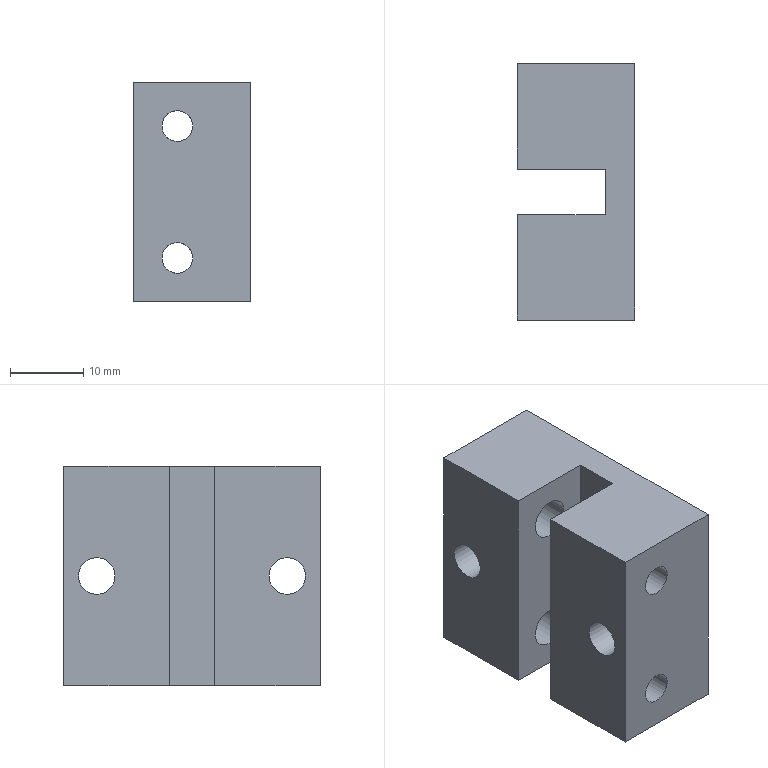Part | NX | features BREP 1 | 1 solid | 20 faces | box 16 x 35 x 30 mm | volume 12265 mm3 | plane 12 | cylinder 8 | commonest cylinder face diameters 4.2 x2 5 x2 5.5 x2 10 x2
STEP:
#1=CARTESIAN_POINT('',(0.1,-3.1,-9.));
#2=VERTEX_POINT('',#1);
#3=CARTESIAN_POINT('',(-2.,-3.1,-9.));
#4=DIRECTION('',(0.,1.,0.));
#5=DIRECTION('',(1.,0.,0.));
#6=AXIS2_PLACEMENT_3D('',#3,#4,#5);
#7=CIRCLE('',#6,2.1);
#8=EDGE_CURVE('',#2,#2,#7,.T.);
#9=ORIENTED_EDGE('',*,*,#8,.F.);
#10=EDGE_LOOP('',(#9));
#11=FACE_BOUND('',#10,.T.);
#12=CARTESIAN_POINT('',(-8.,-3.1,-15.));
#13=VERTEX_POINT('',#12);
#14=CARTESIAN_POINT('',(-8.,-3.1,15.));
#15=VERTEX_POINT('',#14);
#16=CARTESIAN_POINT('',(-8.,-3.1,-28.507));
#17=DIRECTION('',(0.,0.,1.));
#18=VECTOR('',#17,1000.);
#19=LINE('',#16,#18);
#20=EDGE_CURVE('',#13,#15,#19,.T.);
#21=ORIENTED_EDGE('',*,*,#20,.T.);
#22=CARTESIAN_POINT('',(4.,-3.1,15.));
#23=VERTEX_POINT('',#22);
#24=CARTESIAN_POINT('',(-8.,-3.1,15.));
#25=DIRECTION('',(1.,0.,0.));
#26=VECTOR('',#25,1000.);
#27=LINE('',#24,#26);
#28=EDGE_CURVE('',#15,#23,#27,.T.);
#29=ORIENTED_EDGE('',*,*,#28,.T.);
#30=CARTESIAN_POINT('',(4.,-3.1,-15.));
#31=VERTEX_POINT('',#30);
#32=CARTESIAN_POINT('',(4.,-3.1,-28.507));
#33=DIRECTION('',(0.,0.,1.));
#34=VECTOR('',#33,1000.);
#35=LINE('',#32,#34);
#36=EDGE_CURVE('',#31,#23,#35,.T.);
#37=ORIENTED_EDGE('',*,*,#36,.F.);
#38=CARTESIAN_POINT('',(-8.,-3.1,-15.));
#39=DIRECTION('',(1.,0.,0.));
#40=VECTOR('',#39,1000.);
#41=LINE('',#38,#40);
#42=EDGE_CURVE('',#13,#31,#41,.T.);
#43=ORIENTED_EDGE('',*,*,#42,.F.);
#44=EDGE_LOOP('',(#21,#29,#37,#43));
#45=FACE_BOUND('',#44,.T.);
#46=CARTESIAN_POINT('',(0.1,-3.1,9.));
#47=VERTEX_POINT('',#46);
#48=CARTESIAN_POINT('',(-2.,-3.1,9.));
#49=DIRECTION('',(0.,1.,0.));
#50=DIRECTION('',(1.,0.,0.));
#51=AXIS2_PLACEMENT_3D('',#48,#49,#50);
#52=CIRCLE('',#51,2.1);
#53=EDGE_CURVE('',#47,#47,#52,.T.);
#54=ORIENTED_EDGE('',*,*,#53,.F.);
#55=EDGE_LOOP('',(#54));
#56=FACE_BOUND('',#55,.T.);
#57=CARTESIAN_POINT('',(-8.,-3.1,-28.507));
#58=DIRECTION('',(0.,-1.,0.));
#59=DIRECTION('',(-1.,0.,0.));
#60=AXIS2_PLACEMENT_3D('',#57,#58,#59);
#61=PLANE('',#60);
#62=ADVANCED_FACE('',(#11,#45,#56),#61,.F.);
#63=CARTESIAN_POINT('',(-4.75,3.1,9.));
#64=VERTEX_POINT('',#63);
#65=CARTESIAN_POINT('',(-2.,3.1,9.));
#66=DIRECTION('',(0.,-1.,0.));
#67=DIRECTION('',(-1.,0.,0.));
#68=AXIS2_PLACEMENT_3D('',#65,#66,#67);
#69=CIRCLE('',#68,2.75);
#70=EDGE_CURVE('',#64,#64,#69,.T.);
#71=ORIENTED_EDGE('',*,*,#70,.F.);
#72=EDGE_LOOP('',(#71));
#73=FACE_BOUND('',#72,.T.);
#74=CARTESIAN_POINT('',(4.,3.1,-15.));
#75=VERTEX_POINT('',#74);
#76=CARTESIAN_POINT('',(4.,3.1,15.));
#77=VERTEX_POINT('',#76);
#78=CARTESIAN_POINT('',(4.,3.1,-28.507));
#79=DIRECTION('',(0.,0.,1.));
#80=VECTOR('',#79,1000.);
#81=LINE('',#78,#80);
#82=EDGE_CURVE('',#75,#77,#81,.T.);
#83=ORIENTED_EDGE('',*,*,#82,.T.);
#84=CARTESIAN_POINT('',(-8.,3.1,15.));
#85=VERTEX_POINT('',#84);
#86=CARTESIAN_POINT('',(-8.,3.1,15.));
#87=DIRECTION('',(-1.,0.,0.));
#88=VECTOR('',#87,1000.);
#89=LINE('',#86,#88);
#90=EDGE_CURVE('',#77,#85,#89,.T.);
#91=ORIENTED_EDGE('',*,*,#90,.T.);
#92=CARTESIAN_POINT('',(-8.,3.1,-15.));
#93=VERTEX_POINT('',#92);
#94=CARTESIAN_POINT('',(-8.,3.1,-28.507));
#95=DIRECTION('',(0.,0.,1.));
#96=VECTOR('',#95,1000.);
#97=LINE('',#94,#96);
#98=EDGE_CURVE('',#93,#85,#97,.T.);
#99=ORIENTED_EDGE('',*,*,#98,.F.);
#100=CARTESIAN_POINT('',(-8.,3.1,-15.));
#101=DIRECTION('',(-1.,0.,0.));
#102=VECTOR('',#101,1000.);
#103=LINE('',#100,#102);
#104=EDGE_CURVE('',#75,#93,#103,.T.);
#105=ORIENTED_EDGE('',*,*,#104,.F.);
#106=EDGE_LOOP('',(#83,#91,#99,#105));
#107=FACE_BOUND('',#106,.T.);
#108=CARTESIAN_POINT('',(-4.75,3.1,-9.));
#109=VERTEX_POINT('',#108);
#110=CARTESIAN_POINT('',(-2.,3.1,-9.));
#111=DIRECTION('',(0.,-1.,0.));
#112=DIRECTION('',(-1.,0.,0.));
#113=AXIS2_PLACEMENT_3D('',#110,#111,#112);
#114=CIRCLE('',#113,2.75);
#115=EDGE_CURVE('',#109,#109,#114,.T.);
#116=ORIENTED_EDGE('',*,*,#115,.F.);
#117=EDGE_LOOP('',(#116));
#118=FACE_BOUND('',#117,.T.);
#119=CARTESIAN_POINT('',(-8.,3.1,-28.507));
#120=DIRECTION('',(0.,1.,0.));
#121=DIRECTION('',(1.,0.,0.));
#122=AXIS2_PLACEMENT_3D('',#119,#120,#121);
#123=PLANE('',#122);
#124=ADVANCED_FACE('',(#73,#107,#118),#123,.F.);
#125=CARTESIAN_POINT('',(-8.,-13.,-2.5));
#126=VERTEX_POINT('',#125);
#127=CARTESIAN_POINT('',(-8.,-13.,0.));
#128=DIRECTION('',(1.,0.,0.));
#129=DIRECTION('',(0.,0.,-1.));
#130=AXIS2_PLACEMENT_3D('',#127,#128,#129);
#131=CIRCLE('',#130,2.5);
#132=EDGE_CURVE('',#126,#126,#131,.T.);
#133=ORIENTED_EDGE('',*,*,#132,.T.);
#134=EDGE_LOOP('',(#133));
#135=FACE_BOUND('',#134,.T.);
#136=CARTESIAN_POINT('',(-8.,-17.5,15.));
#137=VERTEX_POINT('',#136);
#138=CARTESIAN_POINT('',(-8.,-17.5,15.));
#139=DIRECTION('',(0.,-1.,0.));
#140=VECTOR('',#139,1000.);
#141=LINE('',#138,#140);
#142=EDGE_CURVE('',#15,#137,#141,.T.);
#143=ORIENTED_EDGE('',*,*,#142,.F.);
#144=ORIENTED_EDGE('',*,*,#20,.F.);
#145=CARTESIAN_POINT('',(-8.,-17.5,-15.));
#146=VERTEX_POINT('',#145);
#147=CARTESIAN_POINT('',(-8.,-17.5,-15.));
#148=DIRECTION('',(0.,-1.,0.));
#149=VECTOR('',#148,1000.);
#150=LINE('',#147,#149);
#151=EDGE_CURVE('',#13,#146,#150,.T.);
#152=ORIENTED_EDGE('',*,*,#151,.T.);
#153=CARTESIAN_POINT('',(-8.,-17.5,15.));
#154=DIRECTION('',(0.,0.,-1.));
#155=VECTOR('',#154,1000.);
#156=LINE('',#153,#155);
#157=EDGE_CURVE('',#137,#146,#156,.T.);
#158=ORIENTED_EDGE('',*,*,#157,.F.);
#159=EDGE_LOOP('',(#143,#144,#152,#158));
#160=FACE_BOUND('',#159,.T.);
#161=CARTESIAN_POINT('',(-8.,-17.5,15.));
#162=DIRECTION('',(1.,0.,0.));
#163=DIRECTION('',(0.,0.,1.));
#164=AXIS2_PLACEMENT_3D('',#161,#162,#163);
#165=PLANE('',#164);
#166=ADVANCED_FACE('',(#135,#160),#165,.F.);
#167=CARTESIAN_POINT('',(8.,13.,-2.5));
#168=VERTEX_POINT('',#167);
#169=CARTESIAN_POINT('',(8.,13.,0.));
#170=DIRECTION('',(1.,0.,0.));
#171=DIRECTION('',(0.,0.,-1.));
#172=AXIS2_PLACEMENT_3D('',#169,#170,#171);
#173=CIRCLE('',#172,2.5);
#174=EDGE_CURVE('',#168,#168,#173,.T.);
#175=ORIENTED_EDGE('',*,*,#174,.F.);
#176=EDGE_LOOP('',(#175));
#177=FACE_BOUND('',#176,.T.);
#178=CARTESIAN_POINT('',(8.,-13.,-2.5));
#179=VERTEX_POINT('',#178);
#180=CARTESIAN_POINT('',(8.,-13.,0.));
#181=DIRECTION('',(1.,0.,0.));
#182=DIRECTION('',(0.,0.,-1.));
#183=AXIS2_PLACEMENT_3D('',#180,#181,#182);
#184=CIRCLE('',#183,2.5);
#185=EDGE_CURVE('',#179,#179,#184,.T.);
#186=ORIENTED_EDGE('',*,*,#185,.F.);
#187=EDGE_LOOP('',(#186));
#188=FACE_BOUND('',#187,.T.);
#189=CARTESIAN_POINT('',(8.,-17.5,-15.));
#190=VERTEX_POINT('',#189);
#191=CARTESIAN_POINT('',(8.,17.5,-15.));
#192=VERTEX_POINT('',#191);
#193=CARTESIAN_POINT('',(8.,-17.5,-15.));
#194=DIRECTION('',(0.,1.,0.));
#195=VECTOR('',#194,1000.);
#196=LINE('',#193,#195);
#197=EDGE_CURVE('',#190,#192,#196,.T.);
#198=ORIENTED_EDGE('',*,*,#197,.T.);
#199=CARTESIAN_POINT('',(8.,17.5,15.));
#200=VERTEX_POINT('',#199);
#201=CARTESIAN_POINT('',(8.,17.5,15.));
#202=DIRECTION('',(0.,0.,-1.));
#203=VECTOR('',#202,1000.);
#204=LINE('',#201,#203);
#205=EDGE_CURVE('',#200,#192,#204,.T.);
#206=ORIENTED_EDGE('',*,*,#205,.F.);
#207=CARTESIAN_POINT('',(8.,-17.5,15.));
#208=VERTEX_POINT('',#207);
#209=CARTESIAN_POINT('',(8.,-17.5,15.));
#210=DIRECTION('',(0.,1.,0.));
#211=VECTOR('',#210,1000.);
#212=LINE('',#209,#211);
#213=EDGE_CURVE('',#208,#200,#212,.T.);
#214=ORIENTED_EDGE('',*,*,#213,.F.);
#215=CARTESIAN_POINT('',(8.,-17.5,15.));
#216=DIRECTION('',(0.,0.,-1.));
#217=VECTOR('',#216,1000.);
#218=LINE('',#215,#217);
#219=EDGE_CURVE('',#208,#190,#218,.T.);
#220=ORIENTED_EDGE('',*,*,#219,.T.);
#221=EDGE_LOOP('',(#198,#206,#214,#220));
#222=FACE_BOUND('',#221,.T.);
#223=CARTESIAN_POINT('',(8.,-17.5,15.));
#224=DIRECTION('',(-1.,0.,0.));
#225=DIRECTION('',(0.,0.,-1.));
#226=AXIS2_PLACEMENT_3D('',#223,#224,#225);
#227=PLANE('',#226);
#228=ADVANCED_FACE('',(#177,#188,#222),#227,.F.);
#229=CARTESIAN_POINT('',(-2.,17.5,-4.));
#230=VERTEX_POINT('',#229);
#231=CARTESIAN_POINT('',(-2.,17.5,-9.));
#232=DIRECTION('',(0.,1.,0.));
#233=DIRECTION('',(0.,0.,1.));
#234=AXIS2_PLACEMENT_3D('',#231,#232,#233);
#235=CIRCLE('',#234,5.);
#236=EDGE_CURVE('',#230,#230,#235,.T.);
#237=ORIENTED_EDGE('',*,*,#236,.F.);
#238=EDGE_LOOP('',(#237));
#239=FACE_BOUND('',#238,.T.);
#240=CARTESIAN_POINT('',(-2.,17.5,14.));
#241=VERTEX_POINT('',#240);
#242=CARTESIAN_POINT('',(-2.,17.5,9.));
#243=DIRECTION('',(0.,1.,0.));
#244=DIRECTION('',(0.,0.,1.));
#245=AXIS2_PLACEMENT_3D('',#242,#243,#244);
#246=CIRCLE('',#245,5.);
#247=EDGE_CURVE('',#241,#241,#246,.T.);
#248=ORIENTED_EDGE('',*,*,#247,.F.);
#249=EDGE_LOOP('',(#248));
#250=FACE_BOUND('',#249,.T.);
#251=CARTESIAN_POINT('',(-8.,17.5,-15.));
#252=VERTEX_POINT('',#251);
#253=CARTESIAN_POINT('',(-8.,17.5,-15.));
#254=DIRECTION('',(-1.,0.,0.));
#255=VECTOR('',#254,1000.);
#256=LINE('',#253,#255);
#257=EDGE_CURVE('',#192,#252,#256,.T.);
#258=ORIENTED_EDGE('',*,*,#257,.T.);
#259=CARTESIAN_POINT('',(-8.,17.5,15.));
#260=VERTEX_POINT('',#259);
#261=CARTESIAN_POINT('',(-8.,17.5,15.));
#262=DIRECTION('',(0.,0.,-1.));
#263=VECTOR('',#262,1000.);
#264=LINE('',#261,#263);
#265=EDGE_CURVE('',#260,#252,#264,.T.);
#266=ORIENTED_EDGE('',*,*,#265,.F.);
#267=CARTESIAN_POINT('',(-8.,17.5,15.));
#268=DIRECTION('',(-1.,0.,0.));
#269=VECTOR('',#268,1000.);
#270=LINE('',#267,#269);
#271=EDGE_CURVE('',#200,#260,#270,.T.);
#272=ORIENTED_EDGE('',*,*,#271,.F.);
#273=ORIENTED_EDGE('',*,*,#205,.T.);
#274=EDGE_LOOP('',(#258,#266,#272,#273));
#275=FACE_BOUND('',#274,.T.);
#276=CARTESIAN_POINT('',(-8.,17.5,15.));
#277=DIRECTION('',(0.,-1.,0.));
#278=DIRECTION('',(0.,0.,1.));
#279=AXIS2_PLACEMENT_3D('',#276,#277,#278);
#280=PLANE('',#279);
#281=ADVANCED_FACE('',(#239,#250,#275),#280,.F.);
#282=CARTESIAN_POINT('',(-8.,13.,-2.5));
#283=VERTEX_POINT('',#282);
#284=CARTESIAN_POINT('',(-8.,13.,0.));
#285=DIRECTION('',(1.,0.,0.));
#286=DIRECTION('',(0.,0.,-1.));
#287=AXIS2_PLACEMENT_3D('',#284,#285,#286);
#288=CIRCLE('',#287,2.5);
#289=EDGE_CURVE('',#283,#283,#288,.T.);
#290=ORIENTED_EDGE('',*,*,#289,.T.);
#291=EDGE_LOOP('',(#290));
#292=FACE_BOUND('',#291,.T.);
#293=CARTESIAN_POINT('',(-8.,-17.5,-15.));
#294=DIRECTION('',(0.,-1.,0.));
#295=VECTOR('',#294,1000.);
#296=LINE('',#293,#295);
#297=EDGE_CURVE('',#252,#93,#296,.T.);
#298=ORIENTED_EDGE('',*,*,#297,.T.);
#299=ORIENTED_EDGE('',*,*,#98,.T.);
#300=CARTESIAN_POINT('',(-8.,-17.5,15.));
#301=DIRECTION('',(0.,-1.,0.));
#302=VECTOR('',#301,1000.);
#303=LINE('',#300,#302);
#304=EDGE_CURVE('',#260,#85,#303,.T.);
#305=ORIENTED_EDGE('',*,*,#304,.F.);
#306=ORIENTED_EDGE('',*,*,#265,.T.);
#307=EDGE_LOOP('',(#298,#299,#305,#306));
#308=FACE_BOUND('',#307,.T.);
#309=CARTESIAN_POINT('',(-8.,-17.5,15.));
#310=DIRECTION('',(1.,0.,0.));
#311=DIRECTION('',(0.,0.,1.));
#312=AXIS2_PLACEMENT_3D('',#309,#310,#311);
#313=PLANE('',#312);
#314=ADVANCED_FACE('',(#292,#308),#313,.F.);
#315=CARTESIAN_POINT('',(-2.,-17.5,6.9));
#316=VERTEX_POINT('',#315);
#317=CARTESIAN_POINT('',(-2.,-17.5,9.));
#318=DIRECTION('',(0.,-1.,0.));
#319=DIRECTION('',(0.,0.,-1.));
#320=AXIS2_PLACEMENT_3D('',#317,#318,#319);
#321=CIRCLE('',#320,2.1);
#322=EDGE_CURVE('',#316,#316,#321,.T.);
#323=ORIENTED_EDGE('',*,*,#322,.F.);
#324=EDGE_LOOP('',(#323));
#325=FACE_BOUND('',#324,.T.);
#326=CARTESIAN_POINT('',(-2.,-17.5,-11.1));
#327=VERTEX_POINT('',#326);
#328=CARTESIAN_POINT('',(-2.,-17.5,-9.));
#329=DIRECTION('',(0.,-1.,0.));
#330=DIRECTION('',(0.,0.,-1.));
#331=AXIS2_PLACEMENT_3D('',#328,#329,#330);
#332=CIRCLE('',#331,2.1);
#333=EDGE_CURVE('',#327,#327,#332,.T.);
#334=ORIENTED_EDGE('',*,*,#333,.F.);
#335=EDGE_LOOP('',(#334));
#336=FACE_BOUND('',#335,.T.);
#337=CARTESIAN_POINT('',(-8.,-17.5,-15.));
#338=DIRECTION('',(1.,0.,0.));
#339=VECTOR('',#338,1000.);
#340=LINE('',#337,#339);
#341=EDGE_CURVE('',#146,#190,#340,.T.);
#342=ORIENTED_EDGE('',*,*,#341,.T.);
#343=ORIENTED_EDGE('',*,*,#219,.F.);
#344=CARTESIAN_POINT('',(-8.,-17.5,15.));
#345=DIRECTION('',(1.,0.,0.));
#346=VECTOR('',#345,1000.);
#347=LINE('',#344,#346);
#348=EDGE_CURVE('',#137,#208,#347,.T.);
#349=ORIENTED_EDGE('',*,*,#348,.F.);
#350=ORIENTED_EDGE('',*,*,#157,.T.);
#351=EDGE_LOOP('',(#342,#343,#349,#350));
#352=FACE_BOUND('',#351,.T.);
#353=CARTESIAN_POINT('',(-8.,-17.5,15.));
#354=DIRECTION('',(0.,1.,0.));
#355=DIRECTION('',(0.,0.,-1.));
#356=AXIS2_PLACEMENT_3D('',#353,#354,#355);
#357=PLANE('',#356);
#358=ADVANCED_FACE('',(#325,#336,#352),#357,.F.);
#359=CARTESIAN_POINT('',(4.,3.1,15.));
#360=DIRECTION('',(0.,1.,0.));
#361=VECTOR('',#360,1000.);
#362=LINE('',#359,#361);
#363=EDGE_CURVE('',#23,#77,#362,.T.);
#364=ORIENTED_EDGE('',*,*,#363,.F.);
#365=ORIENTED_EDGE('',*,*,#28,.F.);
#366=ORIENTED_EDGE('',*,*,#142,.T.);
#367=ORIENTED_EDGE('',*,*,#348,.T.);
#368=ORIENTED_EDGE('',*,*,#213,.T.);
#369=ORIENTED_EDGE('',*,*,#271,.T.);
#370=ORIENTED_EDGE('',*,*,#304,.T.);
#371=ORIENTED_EDGE('',*,*,#90,.F.);
#372=EDGE_LOOP('',(#364,#365,#366,#367,#368,#369,#370,#371));
#373=FACE_BOUND('',#372,.T.);
#374=CARTESIAN_POINT('',(0.,0.,15.));
#375=DIRECTION('',(0.,0.,-1.));
#376=DIRECTION('',(1.,0.,0.));
#377=AXIS2_PLACEMENT_3D('',#374,#375,#376);
#378=PLANE('',#377);
#379=ADVANCED_FACE('',(#373),#378,.F.);
#380=ORIENTED_EDGE('',*,*,#42,.T.);
#381=CARTESIAN_POINT('',(4.,3.1,-15.));
#382=DIRECTION('',(0.,1.,0.));
#383=VECTOR('',#382,1000.);
#384=LINE('',#381,#383);
#385=EDGE_CURVE('',#31,#75,#384,.T.);
#386=ORIENTED_EDGE('',*,*,#385,.T.);
#387=ORIENTED_EDGE('',*,*,#104,.T.);
#388=ORIENTED_EDGE('',*,*,#297,.F.);
#389=ORIENTED_EDGE('',*,*,#257,.F.);
#390=ORIENTED_EDGE('',*,*,#197,.F.);
#391=ORIENTED_EDGE('',*,*,#341,.F.);
#392=ORIENTED_EDGE('',*,*,#151,.F.);
#393=EDGE_LOOP('',(#380,#386,#387,#388,#389,#390,#391,#392));
#394=FACE_BOUND('',#393,.T.);
#395=CARTESIAN_POINT('',(0.,0.,-15.));
#396=DIRECTION('',(0.,0.,-1.));
#397=DIRECTION('',(1.,0.,0.));
#398=AXIS2_PLACEMENT_3D('',#395,#396,#397);
#399=PLANE('',#398);
#400=ADVANCED_FACE('',(#394),#399,.T.);
#401=ORIENTED_EDGE('',*,*,#36,.T.);
#402=ORIENTED_EDGE('',*,*,#363,.T.);
#403=ORIENTED_EDGE('',*,*,#82,.F.);
#404=ORIENTED_EDGE('',*,*,#385,.F.);
#405=EDGE_LOOP('',(#401,#402,#403,#404));
#406=FACE_BOUND('',#405,.T.);
#407=CARTESIAN_POINT('',(4.,3.1,-28.507));
#408=DIRECTION('',(1.,0.,0.));
#409=DIRECTION('',(0.,-1.,0.));
#410=AXIS2_PLACEMENT_3D('',#407,#408,#409);
#411=PLANE('',#410);
#412=ADVANCED_FACE('',(#406),#411,.F.);
#413=ORIENTED_EDGE('',*,*,#132,.F.);
#414=EDGE_LOOP('',(#413));
#415=FACE_BOUND('',#414,.T.);
#416=ORIENTED_EDGE('',*,*,#185,.T.);
#417=EDGE_LOOP('',(#416));
#418=FACE_BOUND('',#417,.T.);
#419=CARTESIAN_POINT('',(8.,-13.,0.));
#420=DIRECTION('',(1.,0.,0.));
#421=DIRECTION('',(0.,0.,1.));
#422=AXIS2_PLACEMENT_3D('',#419,#420,#421);
#423=CYLINDRICAL_SURFACE('',#422,2.5);
#424=ADVANCED_FACE('',(#415,#418),#423,.F.);
#425=ORIENTED_EDGE('',*,*,#289,.F.);
#426=EDGE_LOOP('',(#425));
#427=FACE_BOUND('',#426,.T.);
#428=ORIENTED_EDGE('',*,*,#174,.T.);
#429=EDGE_LOOP('',(#428));
#430=FACE_BOUND('',#429,.T.);
#431=CARTESIAN_POINT('',(8.,13.,0.));
#432=DIRECTION('',(1.,0.,0.));
#433=DIRECTION('',(0.,0.,1.));
#434=AXIS2_PLACEMENT_3D('',#431,#432,#433);
#435=CYLINDRICAL_SURFACE('',#434,2.5);
#436=ADVANCED_FACE('',(#427,#430),#435,.F.);
#437=ORIENTED_EDGE('',*,*,#70,.T.);
#438=EDGE_LOOP('',(#437));
#439=FACE_BOUND('',#438,.T.);
#440=CARTESIAN_POINT('',(-2.,12.1,11.75));
#441=VERTEX_POINT('',#440);
#442=CARTESIAN_POINT('',(-2.,12.1,9.));
#443=DIRECTION('',(0.,1.,0.));
#444=DIRECTION('',(0.,0.,1.));
#445=AXIS2_PLACEMENT_3D('',#442,#443,#444);
#446=CIRCLE('',#445,2.75);
#447=EDGE_CURVE('',#441,#441,#446,.T.);
#448=ORIENTED_EDGE('',*,*,#447,.T.);
#449=EDGE_LOOP('',(#448));
#450=FACE_BOUND('',#449,.T.);
#451=CARTESIAN_POINT('',(-2.,17.5,9.));
#452=DIRECTION('',(0.,1.,0.));
#453=DIRECTION('',(0.,0.,-1.));
#454=AXIS2_PLACEMENT_3D('',#451,#452,#453);
#455=CYLINDRICAL_SURFACE('',#454,2.75);
#456=ADVANCED_FACE('',(#439,#450),#455,.F.);
#457=ORIENTED_EDGE('',*,*,#447,.F.);
#458=EDGE_LOOP('',(#457));
#459=FACE_BOUND('',#458,.T.);
#460=CARTESIAN_POINT('',(-2.,12.1,14.));
#461=VERTEX_POINT('',#460);
#462=CARTESIAN_POINT('',(-2.,12.1,9.));
#463=DIRECTION('',(0.,1.,0.));
#464=DIRECTION('',(0.,0.,1.));
#465=AXIS2_PLACEMENT_3D('',#462,#463,#464);
#466=CIRCLE('',#465,5.);
#467=EDGE_CURVE('',#461,#461,#466,.T.);
#468=ORIENTED_EDGE('',*,*,#467,.T.);
#469=EDGE_LOOP('',(#468));
#470=FACE_BOUND('',#469,.T.);
#471=CARTESIAN_POINT('',(0.75,12.1,9.));
#472=DIRECTION('',(0.,-1.,0.));
#473=DIRECTION('',(0.,0.,1.));
#474=AXIS2_PLACEMENT_3D('',#471,#472,#473);
#475=PLANE('',#474);
#476=ADVANCED_FACE('',(#459,#470),#475,.F.);
#477=ORIENTED_EDGE('',*,*,#467,.F.);
#478=EDGE_LOOP('',(#477));
#479=FACE_BOUND('',#478,.T.);
#480=ORIENTED_EDGE('',*,*,#247,.T.);
#481=EDGE_LOOP('',(#480));
#482=FACE_BOUND('',#481,.T.);
#483=CARTESIAN_POINT('',(-2.,17.5,9.));
#484=DIRECTION('',(0.,1.,0.));
#485=DIRECTION('',(0.,0.,-1.));
#486=AXIS2_PLACEMENT_3D('',#483,#484,#485);
#487=CYLINDRICAL_SURFACE('',#486,5.);
#488=ADVANCED_FACE('',(#479,#482),#487,.F.);
#489=ORIENTED_EDGE('',*,*,#115,.T.);
#490=EDGE_LOOP('',(#489));
#491=FACE_BOUND('',#490,.T.);
#492=CARTESIAN_POINT('',(-2.,12.1,-6.25));
#493=VERTEX_POINT('',#492);
#494=CARTESIAN_POINT('',(-2.,12.1,-9.));
#495=DIRECTION('',(0.,1.,0.));
#496=DIRECTION('',(0.,0.,1.));
#497=AXIS2_PLACEMENT_3D('',#494,#495,#496);
#498=CIRCLE('',#497,2.75);
#499=EDGE_CURVE('',#493,#493,#498,.T.);
#500=ORIENTED_EDGE('',*,*,#499,.T.);
#501=EDGE_LOOP('',(#500));
#502=FACE_BOUND('',#501,.T.);
#503=CARTESIAN_POINT('',(-2.,17.5,-9.));
#504=DIRECTION('',(0.,1.,0.));
#505=DIRECTION('',(0.,0.,-1.));
#506=AXIS2_PLACEMENT_3D('',#503,#504,#505);
#507=CYLINDRICAL_SURFACE('',#506,2.75);
#508=ADVANCED_FACE('',(#491,#502),#507,.F.);
#509=ORIENTED_EDGE('',*,*,#499,.F.);
#510=EDGE_LOOP('',(#509));
#511=FACE_BOUND('',#510,.T.);
#512=CARTESIAN_POINT('',(-2.,12.1,-4.));
#513=VERTEX_POINT('',#512);
#514=CARTESIAN_POINT('',(-2.,12.1,-9.));
#515=DIRECTION('',(0.,1.,0.));
#516=DIRECTION('',(0.,0.,1.));
#517=AXIS2_PLACEMENT_3D('',#514,#515,#516);
#518=CIRCLE('',#517,5.);
#519=EDGE_CURVE('',#513,#513,#518,.T.);
#520=ORIENTED_EDGE('',*,*,#519,.T.);
#521=EDGE_LOOP('',(#520));
#522=FACE_BOUND('',#521,.T.);
#523=CARTESIAN_POINT('',(0.75,12.1,-9.));
#524=DIRECTION('',(0.,-1.,0.));
#525=DIRECTION('',(0.,0.,1.));
#526=AXIS2_PLACEMENT_3D('',#523,#524,#525);
#527=PLANE('',#526);
#528=ADVANCED_FACE('',(#511,#522),#527,.F.);
#529=ORIENTED_EDGE('',*,*,#519,.F.);
#530=EDGE_LOOP('',(#529));
#531=FACE_BOUND('',#530,.T.);
#532=ORIENTED_EDGE('',*,*,#236,.T.);
#533=EDGE_LOOP('',(#532));
#534=FACE_BOUND('',#533,.T.);
#535=CARTESIAN_POINT('',(-2.,17.5,-9.));
#536=DIRECTION('',(0.,1.,0.));
#537=DIRECTION('',(0.,0.,-1.));
#538=AXIS2_PLACEMENT_3D('',#535,#536,#537);
#539=CYLINDRICAL_SURFACE('',#538,5.);
#540=ADVANCED_FACE('',(#531,#534),#539,.F.);
#541=ORIENTED_EDGE('',*,*,#8,.T.);
#542=EDGE_LOOP('',(#541));
#543=FACE_BOUND('',#542,.T.);
#544=ORIENTED_EDGE('',*,*,#333,.T.);
#545=EDGE_LOOP('',(#544));
#546=FACE_BOUND('',#545,.T.);
#547=CARTESIAN_POINT('',(-2.,-17.5,-9.));
#548=DIRECTION('',(0.,-1.,0.));
#549=DIRECTION('',(0.,0.,1.));
#550=AXIS2_PLACEMENT_3D('',#547,#548,#549);
#551=CYLINDRICAL_SURFACE('',#550,2.1);
#552=ADVANCED_FACE('',(#543,#546),#551,.F.);
#553=ORIENTED_EDGE('',*,*,#53,.T.);
#554=EDGE_LOOP('',(#553));
#555=FACE_BOUND('',#554,.T.);
#556=ORIENTED_EDGE('',*,*,#322,.T.);
#557=EDGE_LOOP('',(#556));
#558=FACE_BOUND('',#557,.T.);
#559=CARTESIAN_POINT('',(-2.,-17.5,9.));
#560=DIRECTION('',(0.,-1.,0.));
#561=DIRECTION('',(0.,0.,1.));
#562=AXIS2_PLACEMENT_3D('',#559,#560,#561);
#563=CYLINDRICAL_SURFACE('',#562,2.1);
#564=ADVANCED_FACE('',(#555,#558),#563,.F.);
#565=CLOSED_SHELL('',(#62,#124,#166,#228,#281,#314,#358,#379,#400,#412,#424,#436,#456,#476,#488,#508,#528,#540,#552,#564));
#566=MANIFOLD_SOLID_BREP('',#565);
#567=(LENGTH_UNIT()NAMED_UNIT(*)SI_UNIT(.MILLI.,.METRE.));
#568=UNCERTAINTY_MEASURE_WITH_UNIT(LENGTH_MEASURE(0.00001),#567,'','');
#569=(NAMED_UNIT(*)PLANE_ANGLE_UNIT()SI_UNIT($,.RADIAN.));
#570=(NAMED_UNIT(*)SI_UNIT($,.STERADIAN.)SOLID_ANGLE_UNIT());
#571=(GEOMETRIC_REPRESENTATION_CONTEXT(3)GLOBAL_UNCERTAINTY_ASSIGNED_CONTEXT((#568))GLOBAL_UNIT_ASSIGNED_CONTEXT((#567,#569,#570))REPRESENTATION_CONTEXT('',''));
#572=ADVANCED_BREP_SHAPE_REPRESENTATION('',(#566),#571);